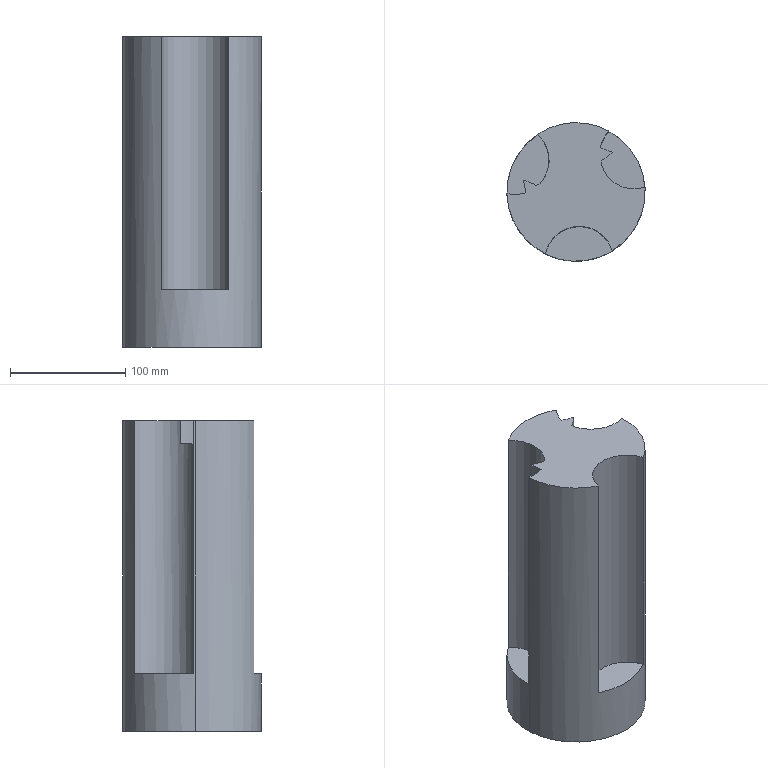Part | SolidWorks | features BaseBody 1 | 1 solid | 18 faces | box 120 x 120 x 270 mm | volume 2222971 mm3 | plane 9 | cylinder 9 | commonest cylinder face diameters 120 x6 60 x3
STEP:
#1=CARTESIAN_POINT('',(231.772,1003.157,-664.893));
#2=VERTEX_POINT('',#1);
#3=CARTESIAN_POINT('',(233.847,960.478,-664.893));
#4=VERTEX_POINT('',#3);
#5=CARTESIAN_POINT('',(211.774,980.794,-664.893));
#6=DIRECTION('',(0.,0.,-1.));
#7=DIRECTION('',(1.,0.,0.));
#8=AXIS2_PLACEMENT_3D('',#5,#6,#7);
#9=CIRCLE('',#8,30.);
#10=EDGE_CURVE('',#2,#4,#9,.T.);
#11=ORIENTED_EDGE('',*,*,#10,.T.);
#12=CARTESIAN_POINT('',(230.967,958.615,-664.893));
#13=VERTEX_POINT('',#12);
#14=CARTESIAN_POINT('',(230.967,958.615,-664.893));
#15=DIRECTION('',(0.8397,0.5431,0.));
#16=VECTOR('',#15,1000.);
#17=LINE('',#14,#16);
#18=EDGE_CURVE('',#13,#4,#17,.T.);
#19=ORIENTED_EDGE('',*,*,#18,.F.);
#20=CARTESIAN_POINT('',(219.47,963.281,-664.893));
#21=VERTEX_POINT('',#20);
#22=CARTESIAN_POINT('',(202.777,905.65,-664.893));
#23=DIRECTION('',(0.,0.,-1.));
#24=DIRECTION('',(1.,0.,0.));
#25=AXIS2_PLACEMENT_3D('',#22,#23,#24);
#26=CIRCLE('',#25,60.);
#27=EDGE_CURVE('',#21,#13,#26,.T.);
#28=ORIENTED_EDGE('',*,*,#27,.F.);
#29=CARTESIAN_POINT('',(221.253,952.331,-664.893));
#30=VERTEX_POINT('',#29);
#31=CARTESIAN_POINT('',(161.395,948.207,-664.893));
#32=DIRECTION('',(0.,0.,-1.));
#33=DIRECTION('',(1.,0.,0.));
#34=AXIS2_PLACEMENT_3D('',#31,#32,#33);
#35=CIRCLE('',#34,60.);
#36=EDGE_CURVE('',#21,#30,#35,.T.);
#37=ORIENTED_EDGE('',*,*,#36,.T.);
#38=CARTESIAN_POINT('',(205.101,951.546,-664.893));
#39=VERTEX_POINT('',#38);
#40=CARTESIAN_POINT('',(211.774,980.794,-664.893));
#41=DIRECTION('',(0.,0.,-1.));
#42=DIRECTION('',(1.,0.,0.));
#43=AXIS2_PLACEMENT_3D('',#40,#41,#42);
#44=CIRCLE('',#43,30.);
#45=EDGE_CURVE('',#30,#39,#44,.T.);
#46=ORIENTED_EDGE('',*,*,#45,.T.);
#47=CARTESIAN_POINT('',(205.142,950.452,-664.893));
#48=VERTEX_POINT('',#47);
#49=CARTESIAN_POINT('',(265.077,953.249,-664.893));
#50=DIRECTION('',(0.,0.,-1.));
#51=DIRECTION('',(1.,0.,0.));
#52=AXIS2_PLACEMENT_3D('',#49,#50,#51);
#53=CIRCLE('',#52,60.);
#54=EDGE_CURVE('',#48,#39,#53,.T.);
#55=ORIENTED_EDGE('',*,*,#54,.F.);
#56=CARTESIAN_POINT('',(238.508,899.452,-664.893));
#57=VERTEX_POINT('',#56);
#58=CARTESIAN_POINT('',(265.077,953.249,-664.893));
#59=DIRECTION('',(0.,0.,-1.));
#60=DIRECTION('',(1.,0.,0.));
#61=AXIS2_PLACEMENT_3D('',#58,#59,#60);
#62=CIRCLE('',#61,60.);
#63=EDGE_CURVE('',#57,#48,#62,.T.);
#64=ORIENTED_EDGE('',*,*,#63,.F.);
#65=CARTESIAN_POINT('',(296.54,902.16,-664.893));
#66=VERTEX_POINT('',#65);
#67=CARTESIAN_POINT('',(267.874,893.314,-664.893));
#68=DIRECTION('',(0.,0.,-1.));
#69=DIRECTION('',(1.,0.,0.));
#70=AXIS2_PLACEMENT_3D('',#67,#68,#69);
#71=CIRCLE('',#70,30.);
#72=EDGE_CURVE('',#57,#66,#71,.T.);
#73=ORIENTED_EDGE('',*,*,#72,.T.);
#74=CARTESIAN_POINT('',(325.012,956.046,-664.893));
#75=VERTEX_POINT('',#74);
#76=CARTESIAN_POINT('',(265.077,953.249,-664.893));
#77=DIRECTION('',(0.,0.,-1.));
#78=DIRECTION('',(1.,0.,0.));
#79=AXIS2_PLACEMENT_3D('',#76,#77,#78);
#80=CIRCLE('',#79,60.);
#81=EDGE_CURVE('',#75,#66,#80,.T.);
#82=ORIENTED_EDGE('',*,*,#81,.F.);
#83=CARTESIAN_POINT('',(324.951,957.138,-664.893));
#84=VERTEX_POINT('',#83);
#85=CARTESIAN_POINT('',(265.077,953.249,-664.893));
#86=DIRECTION('',(0.,0.,-1.));
#87=DIRECTION('',(1.,0.,0.));
#88=AXIS2_PLACEMENT_3D('',#85,#86,#87);
#89=CIRCLE('',#88,60.);
#90=EDGE_CURVE('',#84,#75,#89,.T.);
#91=ORIENTED_EDGE('',*,*,#90,.F.);
#92=CARTESIAN_POINT('',(286.952,976.68,-664.893));
#93=VERTEX_POINT('',#92);
#94=CARTESIAN_POINT('',(315.584,985.638,-664.893));
#95=DIRECTION('',(0.,0.,-1.));
#96=DIRECTION('',(1.,0.,0.));
#97=AXIS2_PLACEMENT_3D('',#94,#95,#96);
#98=CIRCLE('',#97,30.);
#99=EDGE_CURVE('',#84,#93,#98,.T.);
#100=ORIENTED_EDGE('',*,*,#99,.T.);
#101=CARTESIAN_POINT('',(286.779,980.105,-664.893));
#102=VERTEX_POINT('',#101);
#103=CARTESIAN_POINT('',(286.779,980.105,-664.893));
#104=DIRECTION('',(0.05054,-0.9987,0.));
#105=VECTOR('',#104,1000.);
#106=LINE('',#103,#105);
#107=EDGE_CURVE('',#102,#93,#106,.T.);
#108=ORIENTED_EDGE('',*,*,#107,.F.);
#109=CARTESIAN_POINT('',(296.569,987.729,-664.893));
#110=VERTEX_POINT('',#109);
#111=CARTESIAN_POINT('',(255.005,1031.002,-664.893));
#112=DIRECTION('',(0.,0.,-1.));
#113=DIRECTION('',(1.,0.,0.));
#114=AXIS2_PLACEMENT_3D('',#111,#112,#113);
#115=CIRCLE('',#114,60.);
#116=EDGE_CURVE('',#110,#102,#115,.T.);
#117=ORIENTED_EDGE('',*,*,#116,.F.);
#118=CARTESIAN_POINT('',(286.194,991.661,-664.893));
#119=VERTEX_POINT('',#118);
#120=CARTESIAN_POINT('',(312.551,1045.562,-664.893));
#121=DIRECTION('',(0.,0.,-1.));
#122=DIRECTION('',(1.,0.,0.));
#123=AXIS2_PLACEMENT_3D('',#120,#121,#122);
#124=CIRCLE('',#123,60.);
#125=EDGE_CURVE('',#110,#119,#124,.T.);
#126=ORIENTED_EDGE('',*,*,#125,.T.);
#127=CARTESIAN_POINT('',(293.59,1006.041,-664.893));
#128=VERTEX_POINT('',#127);
#129=CARTESIAN_POINT('',(315.584,985.638,-664.893));
#130=DIRECTION('',(0.,0.,-1.));
#131=DIRECTION('',(1.,0.,0.));
#132=AXIS2_PLACEMENT_3D('',#129,#130,#131);
#133=CIRCLE('',#132,30.);
#134=EDGE_CURVE('',#119,#128,#133,.T.);
#135=ORIENTED_EDGE('',*,*,#134,.T.);
#136=CARTESIAN_POINT('',(265.077,953.249,-664.893));
#137=DIRECTION('',(0.,0.,-1.));
#138=DIRECTION('',(1.,0.,0.));
#139=AXIS2_PLACEMENT_3D('',#136,#137,#138);
#140=CIRCLE('',#139,60.);
#141=EDGE_CURVE('',#2,#128,#140,.T.);
#142=ORIENTED_EDGE('',*,*,#141,.F.);
#143=EDGE_LOOP('',(#11,#19,#28,#37,#46,#55,#64,#73,#82,#91,#100,#108,#117,#126,#135,#142));
#144=FACE_OUTER_BOUND('',#143,.T.);
#145=CARTESIAN_POINT('',(265.077,953.249,-664.893));
#146=DIRECTION('',(0.,0.,1.));
#147=DIRECTION('',(1.,0.,0.));
#148=AXIS2_PLACEMENT_3D('',#145,#146,#147);
#149=PLANE('',#148);
#150=ADVANCED_FACE('',(#144),#149,.T.);
#151=CARTESIAN_POINT('',(286.779,980.105,-684.893));
#152=VERTEX_POINT('',#151);
#153=CARTESIAN_POINT('',(286.952,976.68,-684.893));
#154=VERTEX_POINT('',#153);
#155=CARTESIAN_POINT('',(286.779,980.105,-684.893));
#156=DIRECTION('',(0.05054,-0.9987,0.));
#157=VECTOR('',#156,1000.);
#158=LINE('',#155,#157);
#159=EDGE_CURVE('',#152,#154,#158,.T.);
#160=ORIENTED_EDGE('',*,*,#159,.T.);
#161=CARTESIAN_POINT('',(286.194,991.661,-684.893));
#162=VERTEX_POINT('',#161);
#163=CARTESIAN_POINT('',(315.584,985.638,-684.893));
#164=DIRECTION('',(0.,0.,-1.));
#165=DIRECTION('',(0.5398,-0.8418,0.));
#166=AXIS2_PLACEMENT_3D('',#163,#164,#165);
#167=CIRCLE('',#166,30.);
#168=EDGE_CURVE('',#154,#162,#167,.T.);
#169=ORIENTED_EDGE('',*,*,#168,.T.);
#170=CARTESIAN_POINT('',(296.569,987.729,-684.893));
#171=VERTEX_POINT('',#170);
#172=CARTESIAN_POINT('',(312.551,1045.562,-684.893));
#173=DIRECTION('',(0.,0.,-1.));
#174=DIRECTION('',(-0.5,0.866,0.));
#175=AXIS2_PLACEMENT_3D('',#172,#173,#174);
#176=CIRCLE('',#175,60.);
#177=EDGE_CURVE('',#171,#162,#176,.T.);
#178=ORIENTED_EDGE('',*,*,#177,.F.);
#179=CARTESIAN_POINT('',(255.005,1031.002,-684.893));
#180=DIRECTION('',(0.,0.,-1.));
#181=DIRECTION('',(0.9987,0.05054,0.));
#182=AXIS2_PLACEMENT_3D('',#179,#180,#181);
#183=CIRCLE('',#182,60.);
#184=EDGE_CURVE('',#171,#152,#183,.T.);
#185=ORIENTED_EDGE('',*,*,#184,.T.);
#186=EDGE_LOOP('',(#160,#169,#178,#185));
#187=FACE_OUTER_BOUND('',#186,.T.);
#188=CARTESIAN_POINT('',(315.584,985.638,-684.893));
#189=DIRECTION('',(0.,0.,-1.));
#190=DIRECTION('',(0.,-1.,0.));
#191=AXIS2_PLACEMENT_3D('',#188,#189,#190);
#192=PLANE('',#191);
#193=ADVANCED_FACE('',(#187),#192,.T.);
#194=CARTESIAN_POINT('',(324.951,957.138,-884.893));
#195=VERTEX_POINT('',#194);
#196=CARTESIAN_POINT('',(293.59,1006.041,-884.893));
#197=VERTEX_POINT('',#196);
#198=CARTESIAN_POINT('',(315.584,985.638,-884.893));
#199=DIRECTION('',(0.,0.,-1.));
#200=DIRECTION('',(0.5398,-0.8418,0.));
#201=AXIS2_PLACEMENT_3D('',#198,#199,#200);
#202=CIRCLE('',#201,30.);
#203=EDGE_CURVE('',#195,#197,#202,.T.);
#204=ORIENTED_EDGE('',*,*,#203,.F.);
#205=CARTESIAN_POINT('',(265.077,953.249,-884.893));
#206=DIRECTION('',(0.,0.,-1.));
#207=DIRECTION('',(0.5398,-0.8418,0.));
#208=AXIS2_PLACEMENT_3D('',#205,#206,#207);
#209=CIRCLE('',#208,60.);
#210=EDGE_CURVE('',#197,#195,#209,.T.);
#211=ORIENTED_EDGE('',*,*,#210,.F.);
#212=EDGE_LOOP('',(#204,#211));
#213=FACE_OUTER_BOUND('',#212,.T.);
#214=CARTESIAN_POINT('',(315.584,985.638,-884.893));
#215=DIRECTION('',(0.,0.,-1.));
#216=DIRECTION('',(0.,-1.,0.));
#217=AXIS2_PLACEMENT_3D('',#214,#215,#216);
#218=PLANE('',#217);
#219=ADVANCED_FACE('',(#213),#218,.F.);
#220=CARTESIAN_POINT('',(230.967,958.615,-684.893));
#221=VERTEX_POINT('',#220);
#222=CARTESIAN_POINT('',(233.847,960.478,-684.893));
#223=VERTEX_POINT('',#222);
#224=CARTESIAN_POINT('',(230.967,958.615,-684.893));
#225=DIRECTION('',(0.8397,0.5431,0.));
#226=VECTOR('',#225,1000.);
#227=LINE('',#224,#226);
#228=EDGE_CURVE('',#221,#223,#227,.T.);
#229=ORIENTED_EDGE('',*,*,#228,.T.);
#230=CARTESIAN_POINT('',(221.253,952.331,-684.893));
#231=VERTEX_POINT('',#230);
#232=CARTESIAN_POINT('',(211.774,980.794,-684.893));
#233=DIRECTION('',(0.,0.,-1.));
#234=DIRECTION('',(0.4591,0.8884,0.));
#235=AXIS2_PLACEMENT_3D('',#232,#233,#234);
#236=CIRCLE('',#235,30.);
#237=EDGE_CURVE('',#223,#231,#236,.T.);
#238=ORIENTED_EDGE('',*,*,#237,.T.);
#239=CARTESIAN_POINT('',(219.47,963.281,-684.893));
#240=VERTEX_POINT('',#239);
#241=CARTESIAN_POINT('',(161.395,948.207,-684.893));
#242=DIRECTION('',(0.,0.,-1.));
#243=DIRECTION('',(-0.5,-0.866,0.));
#244=AXIS2_PLACEMENT_3D('',#241,#242,#243);
#245=CIRCLE('',#244,60.);
#246=EDGE_CURVE('',#240,#231,#245,.T.);
#247=ORIENTED_EDGE('',*,*,#246,.F.);
#248=CARTESIAN_POINT('',(202.777,905.65,-684.893));
#249=DIRECTION('',(0.,0.,-1.));
#250=DIRECTION('',(-0.5431,0.8397,0.));
#251=AXIS2_PLACEMENT_3D('',#248,#249,#250);
#252=CIRCLE('',#251,60.);
#253=EDGE_CURVE('',#240,#221,#252,.T.);
#254=ORIENTED_EDGE('',*,*,#253,.T.);
#255=EDGE_LOOP('',(#229,#238,#247,#254));
#256=FACE_OUTER_BOUND('',#255,.T.);
#257=CARTESIAN_POINT('',(211.774,980.794,-684.893));
#258=DIRECTION('',(0.,0.,-1.));
#259=DIRECTION('',(0.,-1.,0.));
#260=AXIS2_PLACEMENT_3D('',#257,#258,#259);
#261=PLANE('',#260);
#262=ADVANCED_FACE('',(#256),#261,.T.);
#263=CARTESIAN_POINT('',(231.772,1003.157,-884.893));
#264=VERTEX_POINT('',#263);
#265=CARTESIAN_POINT('',(205.101,951.546,-884.893));
#266=VERTEX_POINT('',#265);
#267=CARTESIAN_POINT('',(211.774,980.794,-884.893));
#268=DIRECTION('',(0.,0.,-1.));
#269=DIRECTION('',(0.4591,0.8884,0.));
#270=AXIS2_PLACEMENT_3D('',#267,#268,#269);
#271=CIRCLE('',#270,30.);
#272=EDGE_CURVE('',#264,#266,#271,.T.);
#273=ORIENTED_EDGE('',*,*,#272,.F.);
#274=CARTESIAN_POINT('',(265.077,953.249,-884.893));
#275=DIRECTION('',(0.,0.,-1.));
#276=DIRECTION('',(0.4591,0.8884,0.));
#277=AXIS2_PLACEMENT_3D('',#274,#275,#276);
#278=CIRCLE('',#277,60.);
#279=EDGE_CURVE('',#266,#264,#278,.T.);
#280=ORIENTED_EDGE('',*,*,#279,.F.);
#281=EDGE_LOOP('',(#273,#280));
#282=FACE_OUTER_BOUND('',#281,.T.);
#283=CARTESIAN_POINT('',(211.774,980.794,-884.893));
#284=DIRECTION('',(0.,0.,-1.));
#285=DIRECTION('',(0.,-1.,0.));
#286=AXIS2_PLACEMENT_3D('',#283,#284,#285);
#287=PLANE('',#286);
#288=ADVANCED_FACE('',(#282),#287,.F.);
#289=CARTESIAN_POINT('',(238.508,899.452,-884.893));
#290=VERTEX_POINT('',#289);
#291=CARTESIAN_POINT('',(296.54,902.16,-884.893));
#292=VERTEX_POINT('',#291);
#293=CARTESIAN_POINT('',(267.874,893.314,-884.893));
#294=DIRECTION('',(0.,0.,-1.));
#295=DIRECTION('',(-0.9989,-0.04661,0.));
#296=AXIS2_PLACEMENT_3D('',#293,#294,#295);
#297=CIRCLE('',#296,30.);
#298=EDGE_CURVE('',#290,#292,#297,.T.);
#299=ORIENTED_EDGE('',*,*,#298,.F.);
#300=CARTESIAN_POINT('',(265.077,953.249,-884.893));
#301=DIRECTION('',(0.,0.,-1.));
#302=DIRECTION('',(-0.9989,-0.04661,0.));
#303=AXIS2_PLACEMENT_3D('',#300,#301,#302);
#304=CIRCLE('',#303,60.);
#305=EDGE_CURVE('',#292,#290,#304,.T.);
#306=ORIENTED_EDGE('',*,*,#305,.F.);
#307=EDGE_LOOP('',(#299,#306));
#308=FACE_OUTER_BOUND('',#307,.T.);
#309=CARTESIAN_POINT('',(267.874,893.314,-884.893));
#310=DIRECTION('',(0.,0.,-1.));
#311=DIRECTION('',(0.,-1.,0.));
#312=AXIS2_PLACEMENT_3D('',#309,#310,#311);
#313=PLANE('',#312);
#314=ADVANCED_FACE('',(#308),#313,.F.);
#315=CARTESIAN_POINT('',(205.142,950.452,-934.893));
#316=VERTEX_POINT('',#315);
#317=CARTESIAN_POINT('',(325.012,956.046,-934.893));
#318=VERTEX_POINT('',#317);
#319=CARTESIAN_POINT('',(265.077,953.249,-934.893));
#320=DIRECTION('',(0.,0.,-1.));
#321=DIRECTION('',(-0.9989,-0.04661,0.));
#322=AXIS2_PLACEMENT_3D('',#319,#320,#321);
#323=CIRCLE('',#322,60.);
#324=EDGE_CURVE('',#316,#318,#323,.T.);
#325=ORIENTED_EDGE('',*,*,#324,.T.);
#326=CARTESIAN_POINT('',(265.077,953.249,-934.893));
#327=DIRECTION('',(0.,0.,-1.));
#328=DIRECTION('',(-0.9989,-0.04661,0.));
#329=AXIS2_PLACEMENT_3D('',#326,#327,#328);
#330=CIRCLE('',#329,60.);
#331=EDGE_CURVE('',#318,#316,#330,.T.);
#332=ORIENTED_EDGE('',*,*,#331,.T.);
#333=EDGE_LOOP('',(#325,#332));
#334=FACE_OUTER_BOUND('',#333,.T.);
#335=CARTESIAN_POINT('',(265.077,953.249,-934.893));
#336=DIRECTION('',(0.,0.,-1.));
#337=DIRECTION('',(0.,-1.,0.));
#338=AXIS2_PLACEMENT_3D('',#335,#336,#337);
#339=PLANE('',#338);
#340=ADVANCED_FACE('',(#334),#339,.T.);
#341=CARTESIAN_POINT('',(325.012,956.046,-934.893));
#342=DIRECTION('',(0.,0.,1.));
#343=VECTOR('',#342,1000.);
#344=LINE('',#341,#343);
#345=EDGE_CURVE('',#318,#75,#344,.T.);
#346=ORIENTED_EDGE('',*,*,#345,.F.);
#347=ORIENTED_EDGE('',*,*,#324,.F.);
#348=CARTESIAN_POINT('',(205.142,950.452,-934.893));
#349=DIRECTION('',(0.,0.,1.));
#350=VECTOR('',#349,1000.);
#351=LINE('',#348,#350);
#352=EDGE_CURVE('',#316,#48,#351,.T.);
#353=ORIENTED_EDGE('',*,*,#352,.T.);
#354=ORIENTED_EDGE('',*,*,#54,.T.);
#355=CARTESIAN_POINT('',(205.101,951.546,-759.893));
#356=DIRECTION('',(0.,0.,1.));
#357=VECTOR('',#356,1000.);
#358=LINE('',#355,#357);
#359=EDGE_CURVE('',#266,#39,#358,.T.);
#360=ORIENTED_EDGE('',*,*,#359,.F.);
#361=ORIENTED_EDGE('',*,*,#279,.T.);
#362=CARTESIAN_POINT('',(231.772,1003.157,-884.893));
#363=DIRECTION('',(0.,0.,1.));
#364=VECTOR('',#363,1000.);
#365=LINE('',#362,#364);
#366=EDGE_CURVE('',#264,#2,#365,.T.);
#367=ORIENTED_EDGE('',*,*,#366,.T.);
#368=ORIENTED_EDGE('',*,*,#141,.T.);
#369=CARTESIAN_POINT('',(293.59,1006.041,-759.893));
#370=DIRECTION('',(0.,0.,1.));
#371=VECTOR('',#370,1000.);
#372=LINE('',#369,#371);
#373=EDGE_CURVE('',#197,#128,#372,.T.);
#374=ORIENTED_EDGE('',*,*,#373,.F.);
#375=ORIENTED_EDGE('',*,*,#210,.T.);
#376=CARTESIAN_POINT('',(324.951,957.138,-884.893));
#377=DIRECTION('',(0.,0.,1.));
#378=VECTOR('',#377,1000.);
#379=LINE('',#376,#378);
#380=EDGE_CURVE('',#195,#84,#379,.T.);
#381=ORIENTED_EDGE('',*,*,#380,.T.);
#382=ORIENTED_EDGE('',*,*,#90,.T.);
#383=EDGE_LOOP('',(#346,#347,#353,#354,#360,#361,#367,#368,#374,#375,#381,#382));
#384=FACE_OUTER_BOUND('',#383,.T.);
#385=CARTESIAN_POINT('',(265.077,953.249,-934.893));
#386=DIRECTION('',(0.,0.,1.));
#387=DIRECTION('',(-0.9989,-0.04661,0.));
#388=AXIS2_PLACEMENT_3D('',#385,#386,#387);
#389=CYLINDRICAL_SURFACE('',#388,60.);
#390=ADVANCED_FACE('',(#384),#389,.T.);
#391=CARTESIAN_POINT('',(286.779,980.105,-634.893));
#392=DIRECTION('',(0.,0.,-1.));
#393=VECTOR('',#392,1000.);
#394=LINE('',#391,#393);
#395=EDGE_CURVE('',#102,#152,#394,.T.);
#396=ORIENTED_EDGE('',*,*,#395,.F.);
#397=ORIENTED_EDGE('',*,*,#107,.T.);
#398=CARTESIAN_POINT('',(286.952,976.68,-634.893));
#399=DIRECTION('',(0.,0.,-1.));
#400=VECTOR('',#399,1000.);
#401=LINE('',#398,#400);
#402=EDGE_CURVE('',#93,#154,#401,.T.);
#403=ORIENTED_EDGE('',*,*,#402,.T.);
#404=ORIENTED_EDGE('',*,*,#159,.F.);
#405=EDGE_LOOP('',(#396,#397,#403,#404));
#406=FACE_OUTER_BOUND('',#405,.T.);
#407=CARTESIAN_POINT('',(286.779,980.105,-634.893));
#408=DIRECTION('',(0.9987,0.05054,0.));
#409=DIRECTION('',(0.,0.,-1.));
#410=AXIS2_PLACEMENT_3D('',#407,#408,#409);
#411=PLANE('',#410);
#412=ADVANCED_FACE('',(#406),#411,.T.);
#413=ORIENTED_EDGE('',*,*,#99,.F.);
#414=ORIENTED_EDGE('',*,*,#380,.F.);
#415=ORIENTED_EDGE('',*,*,#203,.T.);
#416=ORIENTED_EDGE('',*,*,#373,.T.);
#417=ORIENTED_EDGE('',*,*,#134,.F.);
#418=CARTESIAN_POINT('',(286.194,991.661,-884.893));
#419=DIRECTION('',(0.,0.,-1.));
#420=VECTOR('',#419,1000.);
#421=LINE('',#418,#420);
#422=EDGE_CURVE('',#119,#162,#421,.T.);
#423=ORIENTED_EDGE('',*,*,#422,.T.);
#424=ORIENTED_EDGE('',*,*,#168,.F.);
#425=ORIENTED_EDGE('',*,*,#402,.F.);
#426=EDGE_LOOP('',(#413,#414,#415,#416,#417,#423,#424,#425));
#427=FACE_OUTER_BOUND('',#426,.T.);
#428=CARTESIAN_POINT('',(315.584,985.638,-884.893));
#429=DIRECTION('',(0.,0.,1.));
#430=DIRECTION('',(0.9987,0.05054,0.));
#431=AXIS2_PLACEMENT_3D('',#428,#429,#430);
#432=CYLINDRICAL_SURFACE('',#431,30.);
#433=ADVANCED_FACE('',(#427),#432,.F.);
#434=ORIENTED_EDGE('',*,*,#125,.F.);
#435=CARTESIAN_POINT('',(296.569,987.729,-634.893));
#436=DIRECTION('',(0.,0.,-1.));
#437=VECTOR('',#436,1000.);
#438=LINE('',#435,#437);
#439=EDGE_CURVE('',#110,#171,#438,.T.);
#440=ORIENTED_EDGE('',*,*,#439,.T.);
#441=ORIENTED_EDGE('',*,*,#177,.T.);
#442=ORIENTED_EDGE('',*,*,#422,.F.);
#443=EDGE_LOOP('',(#434,#440,#441,#442));
#444=FACE_OUTER_BOUND('',#443,.T.);
#445=CARTESIAN_POINT('',(312.551,1045.562,-884.893));
#446=DIRECTION('',(0.,0.,1.));
#447=DIRECTION('',(0.9987,0.05054,0.));
#448=AXIS2_PLACEMENT_3D('',#445,#446,#447);
#449=CYLINDRICAL_SURFACE('',#448,60.);
#450=ADVANCED_FACE('',(#444),#449,.F.);
#451=ORIENTED_EDGE('',*,*,#439,.F.);
#452=ORIENTED_EDGE('',*,*,#116,.T.);
#453=ORIENTED_EDGE('',*,*,#395,.T.);
#454=ORIENTED_EDGE('',*,*,#184,.F.);
#455=EDGE_LOOP('',(#451,#452,#453,#454));
#456=FACE_OUTER_BOUND('',#455,.T.);
#457=CARTESIAN_POINT('',(255.005,1031.002,-634.893));
#458=DIRECTION('',(0.,0.,-1.));
#459=DIRECTION('',(-0.9987,-0.05054,0.));
#460=AXIS2_PLACEMENT_3D('',#457,#458,#459);
#461=CYLINDRICAL_SURFACE('',#460,60.);
#462=ADVANCED_FACE('',(#456),#461,.T.);
#463=ORIENTED_EDGE('',*,*,#72,.F.);
#464=CARTESIAN_POINT('',(238.508,899.452,-759.893));
#465=DIRECTION('',(0.,0.,1.));
#466=VECTOR('',#465,1000.);
#467=LINE('',#464,#466);
#468=EDGE_CURVE('',#290,#57,#467,.T.);
#469=ORIENTED_EDGE('',*,*,#468,.F.);
#470=ORIENTED_EDGE('',*,*,#298,.T.);
#471=CARTESIAN_POINT('',(296.54,902.16,-759.893));
#472=DIRECTION('',(0.,0.,-1.));
#473=VECTOR('',#472,1000.);
#474=LINE('',#471,#473);
#475=EDGE_CURVE('',#66,#292,#474,.T.);
#476=ORIENTED_EDGE('',*,*,#475,.F.);
#477=EDGE_LOOP('',(#463,#469,#470,#476));
#478=FACE_OUTER_BOUND('',#477,.T.);
#479=CARTESIAN_POINT('',(267.874,893.314,-634.893));
#480=DIRECTION('',(0.,0.,-1.));
#481=DIRECTION('',(0.9989,0.04661,0.));
#482=AXIS2_PLACEMENT_3D('',#479,#480,#481);
#483=CYLINDRICAL_SURFACE('',#482,30.);
#484=ADVANCED_FACE('',(#478),#483,.F.);
#485=CARTESIAN_POINT('',(230.967,958.615,-634.893));
#486=DIRECTION('',(0.,0.,-1.));
#487=VECTOR('',#486,1000.);
#488=LINE('',#485,#487);
#489=EDGE_CURVE('',#13,#221,#488,.T.);
#490=ORIENTED_EDGE('',*,*,#489,.F.);
#491=ORIENTED_EDGE('',*,*,#18,.T.);
#492=CARTESIAN_POINT('',(233.847,960.478,-634.893));
#493=DIRECTION('',(0.,0.,-1.));
#494=VECTOR('',#493,1000.);
#495=LINE('',#492,#494);
#496=EDGE_CURVE('',#4,#223,#495,.T.);
#497=ORIENTED_EDGE('',*,*,#496,.T.);
#498=ORIENTED_EDGE('',*,*,#228,.F.);
#499=EDGE_LOOP('',(#490,#491,#497,#498));
#500=FACE_OUTER_BOUND('',#499,.T.);
#501=CARTESIAN_POINT('',(230.967,958.615,-634.893));
#502=DIRECTION('',(-0.5431,0.8397,0.));
#503=DIRECTION('',(0.,0.,1.));
#504=AXIS2_PLACEMENT_3D('',#501,#502,#503);
#505=PLANE('',#504);
#506=ADVANCED_FACE('',(#500),#505,.T.);
#507=ORIENTED_EDGE('',*,*,#45,.F.);
#508=CARTESIAN_POINT('',(221.253,952.331,-884.893));
#509=DIRECTION('',(0.,0.,-1.));
#510=VECTOR('',#509,1000.);
#511=LINE('',#508,#510);
#512=EDGE_CURVE('',#30,#231,#511,.T.);
#513=ORIENTED_EDGE('',*,*,#512,.T.);
#514=ORIENTED_EDGE('',*,*,#237,.F.);
#515=ORIENTED_EDGE('',*,*,#496,.F.);
#516=ORIENTED_EDGE('',*,*,#10,.F.);
#517=ORIENTED_EDGE('',*,*,#366,.F.);
#518=ORIENTED_EDGE('',*,*,#272,.T.);
#519=ORIENTED_EDGE('',*,*,#359,.T.);
#520=EDGE_LOOP('',(#507,#513,#514,#515,#516,#517,#518,#519));
#521=FACE_OUTER_BOUND('',#520,.T.);
#522=CARTESIAN_POINT('',(211.774,980.794,-884.893));
#523=DIRECTION('',(0.,0.,1.));
#524=DIRECTION('',(-0.5431,0.8397,0.));
#525=AXIS2_PLACEMENT_3D('',#522,#523,#524);
#526=CYLINDRICAL_SURFACE('',#525,30.);
#527=ADVANCED_FACE('',(#521),#526,.F.);
#528=ORIENTED_EDGE('',*,*,#36,.F.);
#529=CARTESIAN_POINT('',(219.47,963.281,-634.893));
#530=DIRECTION('',(0.,0.,-1.));
#531=VECTOR('',#530,1000.);
#532=LINE('',#529,#531);
#533=EDGE_CURVE('',#21,#240,#532,.T.);
#534=ORIENTED_EDGE('',*,*,#533,.T.);
#535=ORIENTED_EDGE('',*,*,#246,.T.);
#536=ORIENTED_EDGE('',*,*,#512,.F.);
#537=EDGE_LOOP('',(#528,#534,#535,#536));
#538=FACE_OUTER_BOUND('',#537,.T.);
#539=CARTESIAN_POINT('',(161.395,948.207,-884.893));
#540=DIRECTION('',(0.,0.,1.));
#541=DIRECTION('',(-0.5431,0.8397,0.));
#542=AXIS2_PLACEMENT_3D('',#539,#540,#541);
#543=CYLINDRICAL_SURFACE('',#542,60.);
#544=ADVANCED_FACE('',(#538),#543,.F.);
#545=ORIENTED_EDGE('',*,*,#533,.F.);
#546=ORIENTED_EDGE('',*,*,#27,.T.);
#547=ORIENTED_EDGE('',*,*,#489,.T.);
#548=ORIENTED_EDGE('',*,*,#253,.F.);
#549=EDGE_LOOP('',(#545,#546,#547,#548));
#550=FACE_OUTER_BOUND('',#549,.T.);
#551=CARTESIAN_POINT('',(202.777,905.65,-634.893));
#552=DIRECTION('',(0.,0.,-1.));
#553=DIRECTION('',(0.5431,-0.8397,0.));
#554=AXIS2_PLACEMENT_3D('',#551,#552,#553);
#555=CYLINDRICAL_SURFACE('',#554,60.);
#556=ADVANCED_FACE('',(#550),#555,.T.);
#557=ORIENTED_EDGE('',*,*,#331,.F.);
#558=ORIENTED_EDGE('',*,*,#345,.T.);
#559=ORIENTED_EDGE('',*,*,#81,.T.);
#560=ORIENTED_EDGE('',*,*,#475,.T.);
#561=ORIENTED_EDGE('',*,*,#305,.T.);
#562=ORIENTED_EDGE('',*,*,#468,.T.);
#563=ORIENTED_EDGE('',*,*,#63,.T.);
#564=ORIENTED_EDGE('',*,*,#352,.F.);
#565=EDGE_LOOP('',(#557,#558,#559,#560,#561,#562,#563,#564));
#566=FACE_OUTER_BOUND('',#565,.T.);
#567=CARTESIAN_POINT('',(265.077,953.249,-934.893));
#568=DIRECTION('',(0.,0.,1.));
#569=DIRECTION('',(-0.9989,-0.04661,0.));
#570=AXIS2_PLACEMENT_3D('',#567,#568,#569);
#571=CYLINDRICAL_SURFACE('',#570,60.);
#572=ADVANCED_FACE('',(#566),#571,.T.);
#573=CLOSED_SHELL('',(#150,#193,#219,#262,#288,#314,#340,#390,#412,#433,#450,#462,#484,#506,#527,#544,#556,#572));
#574=MANIFOLD_SOLID_BREP('',#573);
#575=CARTESIAN_POINT('',(0.,0.,0.));
#576=DIRECTION('',(0.,0.,1.));
#577=DIRECTION('',(1.,0.,0.));
#578=AXIS2_PLACEMENT_3D('',#575,#576,#577);
#579=(LENGTH_UNIT()NAMED_UNIT(*)SI_UNIT(.MILLI.,.METRE.));
#580=UNCERTAINTY_MEASURE_WITH_UNIT(LENGTH_MEASURE(0.00001),#579,'','');
#581=(NAMED_UNIT(*)PLANE_ANGLE_UNIT()SI_UNIT($,.RADIAN.));
#582=(NAMED_UNIT(*)SI_UNIT($,.STERADIAN.)SOLID_ANGLE_UNIT());
#583=(GEOMETRIC_REPRESENTATION_CONTEXT(3)GLOBAL_UNCERTAINTY_ASSIGNED_CONTEXT((#580))GLOBAL_UNIT_ASSIGNED_CONTEXT((#579,#581,#582))REPRESENTATION_CONTEXT('',''));
#584=ADVANCED_BREP_SHAPE_REPRESENTATION('',(#574,#578),#583);